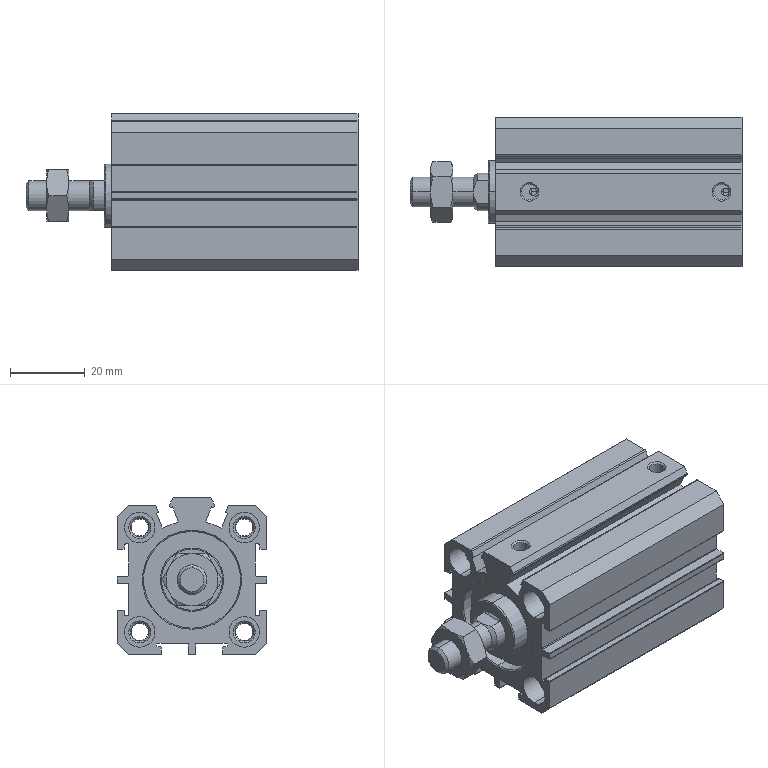Part | SolidWorks | S-SDA25x35-S-B(0_0).stp | 2 solids | 256 faces | box 89 x 40 x 42 mm | volume 65773 mm3 | cylinder 105 | plane 101 | cone 48 | torus 2 | commonest cylinder face diameters 0.4 x36 4.917 x16 8.2 x16 4.6 x8 0.8 x4 2 x4